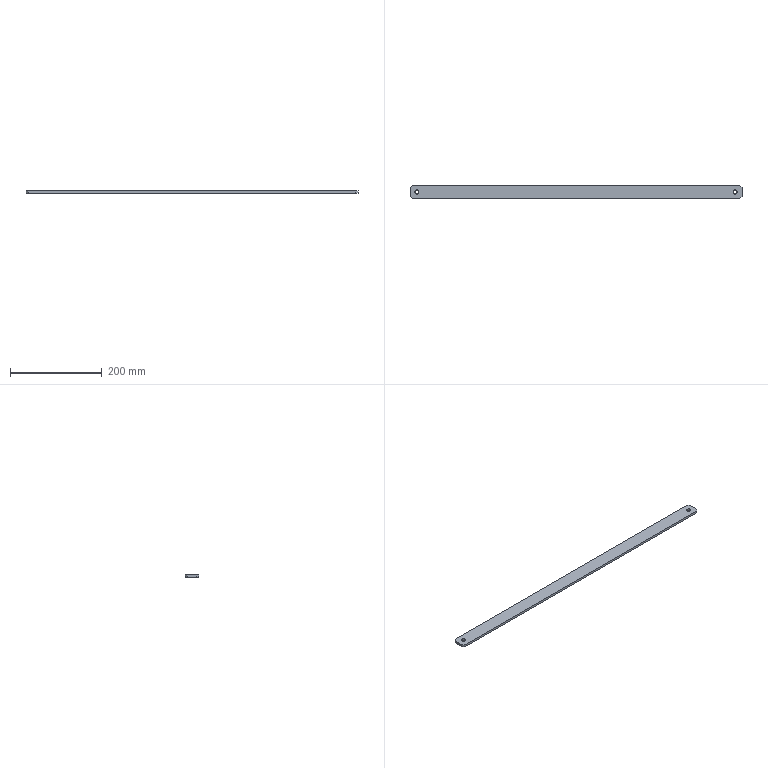Part | STEP file | link-forlegfor roller | 1 solid | 12 faces | box 725.486 x 30 x 5 mm | volume 107937 mm3 | plane 10 | spline 2
STEP:
#1=CARTESIAN_POINT('',(0.,0.,0.));
#2=DIRECTION('',(0.,0.,1.));
#3=DIRECTION('',(1.,0.,0.));
#4=AXIS2_PLACEMENT_3D('',#1,#2,#3);
#5=CARTESIAN_POINT('',(705.986,15.,0.));
#6=VERTEX_POINT('',#5);
#7=CARTESIAN_POINT('',(710.486,15.,0.));
#8=DIRECTION('',(0.,0.,1.));
#9=DIRECTION('',(1.,0.,0.));
#10=AXIS2_PLACEMENT_3D('',#7,#8,#9);
#11=CIRCLE('',#10,4.5);
#12=CARTESIAN_POINT('',(705.986,15.,5.));
#13=CARTESIAN_POINT('',(705.986,10.5,5.));
#14=CARTESIAN_POINT('',(710.486,10.5,5.));
#15=CARTESIAN_POINT('',(714.986,10.5,5.));
#16=CARTESIAN_POINT('',(714.986,15.,5.));
#17=CARTESIAN_POINT('',(714.986,19.5,5.));
#18=CARTESIAN_POINT('',(710.486,19.5,5.));
#19=CARTESIAN_POINT('',(705.986,19.5,5.));
#20=CARTESIAN_POINT('',(705.986,15.,5.));
#21=CARTESIAN_POINT('',(705.986,15.,0.));
#22=CARTESIAN_POINT('',(705.986,10.5,0.));
#23=CARTESIAN_POINT('',(710.486,10.5,0.));
#24=CARTESIAN_POINT('',(714.986,10.5,0.));
#25=CARTESIAN_POINT('',(714.986,15.,0.));
#26=CARTESIAN_POINT('',(714.986,19.5,0.));
#27=CARTESIAN_POINT('',(710.486,19.5,0.));
#28=CARTESIAN_POINT('',(705.986,19.5,0.));
#29=CARTESIAN_POINT('',(705.986,15.,0.));
#30=(BOUNDED_SURFACE()B_SPLINE_SURFACE(1,2,((#12,#13,#14,#15,#16,#17,#18,#19,#20),(#21,#22,#23,#24,#25,#26,#27,#28,#29)),.UNSPECIFIED.,.F.,.T.,.F.)B_SPLINE_SURFACE_WITH_KNOTS((2,2),(1,2,2,2,2,2,1),(-161.361,-160.25),(-7.069,0.,7.069,14.137,21.206,28.274,35.343),.UNSPECIFIED.)GEOMETRIC_REPRESENTATION_ITEM()RATIONAL_B_SPLINE_SURFACE(((1.,0.7071,1.,0.7071,1.,0.7071,1.,0.7071,1.),(1.,0.7071,1.,0.7071,1.,0.7071,1.,0.7071,1.)))REPRESENTATION_ITEM('')SURFACE());
#31=CARTESIAN_POINT('',(-160.25,0.));
#32=CARTESIAN_POINT('',(-160.25,0.4746));
#33=CARTESIAN_POINT('',(-160.25,1.373));
#34=CARTESIAN_POINT('',(-160.25,2.623));
#35=CARTESIAN_POINT('',(-160.25,3.837));
#36=CARTESIAN_POINT('',(-160.25,5.064));
#37=CARTESIAN_POINT('',(-160.25,6.348));
#38=CARTESIAN_POINT('',(-160.25,7.789));
#39=CARTESIAN_POINT('',(-160.25,9.073));
#40=CARTESIAN_POINT('',(-160.25,10.3));
#41=CARTESIAN_POINT('',(-160.25,11.516));
#42=CARTESIAN_POINT('',(-160.25,12.758));
#43=CARTESIAN_POINT('',(-160.25,14.137));
#44=CARTESIAN_POINT('',(-160.25,15.517));
#45=CARTESIAN_POINT('',(-160.25,16.758));
#46=CARTESIAN_POINT('',(-160.25,17.974));
#47=CARTESIAN_POINT('',(-160.25,19.202));
#48=CARTESIAN_POINT('',(-160.25,20.485));
#49=CARTESIAN_POINT('',(-160.25,21.926));
#50=CARTESIAN_POINT('',(-160.25,23.21));
#51=CARTESIAN_POINT('',(-160.25,24.438));
#52=CARTESIAN_POINT('',(-160.25,25.651));
#53=CARTESIAN_POINT('',(-160.25,26.902));
#54=CARTESIAN_POINT('',(-160.25,27.8));
#55=CARTESIAN_POINT('',(-160.25,28.274));
#56=B_SPLINE_CURVE_WITH_KNOTS('',3,(#31,#32,#33,#34,#35,#36,#37,#38,#39,#40,#41,#42,#43,#44,#45,#46,#47,#48,#49,#50,#51,#52,#53,#54,#55),.UNSPECIFIED.,.F.,.F.,(4,1,1,1,1,1,1,1,1,1,1,1,1,1,1,1,1,1,1,1,1,1,4),(3.142,3.427,3.713,3.998,4.284,4.57,4.855,5.141,5.426,5.712,5.998,6.283,6.569,6.854,7.14,7.426,7.711,7.997,8.282,8.568,8.854,9.139,9.425),.QUASI_UNIFORM_KNOTS.);
#57=(GEOMETRIC_REPRESENTATION_CONTEXT(2)PARAMETRIC_REPRESENTATION_CONTEXT()REPRESENTATION_CONTEXT('',''));
#58=DEFINITIONAL_REPRESENTATION('',(#56),#57);
#59=PCURVE('',#30,#58);
#60=CARTESIAN_POINT('',(362.743,15.,0.));
#61=DIRECTION('',(0.,0.,1.));
#62=DIRECTION('',(1.,0.,0.));
#63=AXIS2_PLACEMENT_3D('',#60,#61,#62);
#64=PLANE('',#63);
#65=CARTESIAN_POINT('',(347.743,0.));
#66=DIRECTION('',(1.,0.));
#67=AXIS2_PLACEMENT_2D('',#65,#66);
#68=CIRCLE('',#67,4.5);
#69=(GEOMETRIC_REPRESENTATION_CONTEXT(2)PARAMETRIC_REPRESENTATION_CONTEXT()REPRESENTATION_CONTEXT('',''));
#70=DEFINITIONAL_REPRESENTATION('',(#68),#69);
#71=PCURVE('',#64,#70);
#72=SURFACE_CURVE('',#11,(#59,#71),.PCURVE_S1.);
#73=EDGE_CURVE('',#6,#6,#72,.T.);
#74=ORIENTED_EDGE('',*,*,#73,.T.);
#75=CARTESIAN_POINT('',(705.986,15.,5.));
#76=VERTEX_POINT('',#75);
#77=CARTESIAN_POINT('',(705.986,15.,5.));
#78=CARTESIAN_POINT('',(705.986,15.,0.));
#79=B_SPLINE_CURVE_WITH_KNOTS('',1,(#77,#78),.UNSPECIFIED.,.F.,.F.,(2,2),(-161.361,-160.25),.PIECEWISE_BEZIER_KNOTS.);
#80=CARTESIAN_POINT('',(0.,28.274));
#81=DIRECTION('',(1.,0.));
#82=VECTOR('',#81,1.);
#83=LINE('',#80,#82);
#84=(GEOMETRIC_REPRESENTATION_CONTEXT(2)PARAMETRIC_REPRESENTATION_CONTEXT()REPRESENTATION_CONTEXT('',''));
#85=DEFINITIONAL_REPRESENTATION('',(#83),#84);
#86=PCURVE('',#30,#85);
#87=CARTESIAN_POINT('',(0.,0.));
#88=DIRECTION('',(1.,0.));
#89=VECTOR('',#88,1.);
#90=LINE('',#87,#89);
#91=(GEOMETRIC_REPRESENTATION_CONTEXT(2)PARAMETRIC_REPRESENTATION_CONTEXT()REPRESENTATION_CONTEXT('',''));
#92=DEFINITIONAL_REPRESENTATION('',(#90),#91);
#93=PCURVE('',#30,#92);
#94=SEAM_CURVE('',#79,(#86,#93),.PCURVE_S1.);
#95=EDGE_CURVE('',#76,#6,#94,.T.);
#96=ORIENTED_EDGE('',*,*,#95,.F.);
#97=CARTESIAN_POINT('',(714.986,15.,5.));
#98=VERTEX_POINT('',#97);
#99=CARTESIAN_POINT('',(710.486,15.,5.));
#100=DIRECTION('',(0.,0.,-1.));
#101=DIRECTION('',(1.,0.,0.));
#102=AXIS2_PLACEMENT_3D('',#99,#100,#101);
#103=CIRCLE('',#102,4.5);
#104=CARTESIAN_POINT('',(-161.361,42.412));
#105=CARTESIAN_POINT('',(-161.361,41.937));
#106=CARTESIAN_POINT('',(-161.361,41.039));
#107=CARTESIAN_POINT('',(-161.361,39.788));
#108=CARTESIAN_POINT('',(-161.361,38.575));
#109=CARTESIAN_POINT('',(-161.361,37.347));
#110=CARTESIAN_POINT('',(-161.361,36.064));
#111=CARTESIAN_POINT('',(-161.361,34.622));
#112=CARTESIAN_POINT('',(-161.361,33.339));
#113=CARTESIAN_POINT('',(-161.361,32.111));
#114=CARTESIAN_POINT('',(-161.361,30.896));
#115=CARTESIAN_POINT('',(-161.361,29.654));
#116=CARTESIAN_POINT('',(-161.361,28.274));
#117=CARTESIAN_POINT('',(-161.361,26.895));
#118=CARTESIAN_POINT('',(-161.361,25.653));
#119=CARTESIAN_POINT('',(-161.361,24.437));
#120=CARTESIAN_POINT('',(-161.361,23.21));
#121=CARTESIAN_POINT('',(-161.361,21.926));
#122=CARTESIAN_POINT('',(-161.361,20.485));
#123=CARTESIAN_POINT('',(-161.361,19.202));
#124=CARTESIAN_POINT('',(-161.361,17.974));
#125=CARTESIAN_POINT('',(-161.361,16.76));
#126=CARTESIAN_POINT('',(-161.361,15.51));
#127=CARTESIAN_POINT('',(-161.361,14.612));
#128=CARTESIAN_POINT('',(-161.361,14.137));
#129=B_SPLINE_CURVE_WITH_KNOTS('',3,(#104,#105,#106,#107,#108,#109,#110,#111,#112,#113,#114,#115,#116,#117,#118,#119,#120,#121,#122,#123,#124,#125,#126,#127,#128),.UNSPECIFIED.,.F.,.F.,(4,1,1,1,1,1,1,1,1,1,1,1,1,1,1,1,1,1,1,1,1,1,4),(0.,0.2856,0.5712,0.8568,1.142,1.428,1.714,1.999,2.285,2.57,2.856,3.142,3.427,3.713,3.998,4.284,4.57,4.855,5.141,5.426,5.712,5.998,6.283),.QUASI_UNIFORM_KNOTS.);
#130=(GEOMETRIC_REPRESENTATION_CONTEXT(2)PARAMETRIC_REPRESENTATION_CONTEXT()REPRESENTATION_CONTEXT('',''));
#131=DEFINITIONAL_REPRESENTATION('',(#129),#130);
#132=PCURVE('',#30,#131);
#133=CARTESIAN_POINT('',(362.743,15.,5.));
#134=DIRECTION('',(0.,0.,1.));
#135=DIRECTION('',(1.,0.,0.));
#136=AXIS2_PLACEMENT_3D('',#133,#134,#135);
#137=PLANE('',#136);
#138=CARTESIAN_POINT('',(352.243,0.));
#139=CARTESIAN_POINT('',(352.243,-7.794));
#140=CARTESIAN_POINT('',(345.493,-3.897));
#141=CARTESIAN_POINT('',(338.743,0.));
#142=CARTESIAN_POINT('',(345.493,3.897));
#143=CARTESIAN_POINT('',(352.243,7.794));
#144=CARTESIAN_POINT('',(352.243,0.));
#145=(BOUNDED_CURVE()B_SPLINE_CURVE(2,(#138,#139,#140,#141,#142,#143,#144),.UNSPECIFIED.,.T.,.F.)B_SPLINE_CURVE_WITH_KNOTS((1,2,2,2,2,1),(-2.094,0.,2.094,4.189,6.283,8.378),.UNSPECIFIED.)CURVE()GEOMETRIC_REPRESENTATION_ITEM()RATIONAL_B_SPLINE_CURVE((1.,0.5,1.,0.5,1.,0.5,1.))REPRESENTATION_ITEM(''));
#146=(GEOMETRIC_REPRESENTATION_CONTEXT(2)PARAMETRIC_REPRESENTATION_CONTEXT()REPRESENTATION_CONTEXT('',''));
#147=DEFINITIONAL_REPRESENTATION('',(#145),#146);
#148=PCURVE('',#137,#147);
#149=SURFACE_CURVE('',#103,(#132,#148),.PCURVE_S1.);
#150=EDGE_CURVE('',#76,#98,#149,.T.);
#151=ORIENTED_EDGE('',*,*,#150,.T.);
#152=CARTESIAN_POINT('',(710.486,15.,5.));
#153=DIRECTION('',(0.,0.,-1.));
#154=DIRECTION('',(1.,0.,0.));
#155=AXIS2_PLACEMENT_3D('',#152,#153,#154);
#156=CIRCLE('',#155,4.5);
#157=CARTESIAN_POINT('',(-161.361,14.137));
#158=CARTESIAN_POINT('',(-161.361,13.663));
#159=CARTESIAN_POINT('',(-161.361,12.765));
#160=CARTESIAN_POINT('',(-161.361,11.514));
#161=CARTESIAN_POINT('',(-161.361,10.301));
#162=CARTESIAN_POINT('',(-161.361,9.073));
#163=CARTESIAN_POINT('',(-161.361,7.789));
#164=CARTESIAN_POINT('',(-161.361,6.348));
#165=CARTESIAN_POINT('',(-161.361,5.064));
#166=CARTESIAN_POINT('',(-161.361,3.837));
#167=CARTESIAN_POINT('',(-161.361,2.621));
#168=CARTESIAN_POINT('',(-161.361,1.379));
#169=CARTESIAN_POINT('',(-161.361,0.));
#170=CARTESIAN_POINT('',(-161.361,-1.379));
#171=CARTESIAN_POINT('',(-161.361,-2.621));
#172=CARTESIAN_POINT('',(-161.361,-3.837));
#173=CARTESIAN_POINT('',(-161.361,-5.064));
#174=CARTESIAN_POINT('',(-161.361,-6.348));
#175=CARTESIAN_POINT('',(-161.361,-7.789));
#176=CARTESIAN_POINT('',(-161.361,-9.073));
#177=CARTESIAN_POINT('',(-161.361,-10.301));
#178=CARTESIAN_POINT('',(-161.361,-11.514));
#179=CARTESIAN_POINT('',(-161.361,-12.765));
#180=CARTESIAN_POINT('',(-161.361,-13.663));
#181=CARTESIAN_POINT('',(-161.361,-14.137));
#182=B_SPLINE_CURVE_WITH_KNOTS('',3,(#157,#158,#159,#160,#161,#162,#163,#164,#165,#166,#167,#168,#169,#170,#171,#172,#173,#174,#175,#176,#177,#178,#179,#180,#181),.UNSPECIFIED.,.F.,.F.,(4,1,1,1,1,1,1,1,1,1,1,1,1,1,1,1,1,1,1,1,1,1,4),(0.,0.2856,0.5712,0.8568,1.142,1.428,1.714,1.999,2.285,2.57,2.856,3.142,3.427,3.713,3.998,4.284,4.57,4.855,5.141,5.426,5.712,5.998,6.283),.QUASI_UNIFORM_KNOTS.);
#183=(GEOMETRIC_REPRESENTATION_CONTEXT(2)PARAMETRIC_REPRESENTATION_CONTEXT()REPRESENTATION_CONTEXT('',''));
#184=DEFINITIONAL_REPRESENTATION('',(#182),#183);
#185=PCURVE('',#30,#184);
#186=CARTESIAN_POINT('',(352.243,0.));
#187=CARTESIAN_POINT('',(352.243,-7.794));
#188=CARTESIAN_POINT('',(345.493,-3.897));
#189=CARTESIAN_POINT('',(338.743,0.));
#190=CARTESIAN_POINT('',(345.493,3.897));
#191=CARTESIAN_POINT('',(352.243,7.794));
#192=CARTESIAN_POINT('',(352.243,0.));
#193=(BOUNDED_CURVE()B_SPLINE_CURVE(2,(#186,#187,#188,#189,#190,#191,#192),.UNSPECIFIED.,.T.,.F.)B_SPLINE_CURVE_WITH_KNOTS((1,2,2,2,2,1),(-2.094,0.,2.094,4.189,6.283,8.378),.UNSPECIFIED.)CURVE()GEOMETRIC_REPRESENTATION_ITEM()RATIONAL_B_SPLINE_CURVE((1.,0.5,1.,0.5,1.,0.5,1.))REPRESENTATION_ITEM(''));
#194=(GEOMETRIC_REPRESENTATION_CONTEXT(2)PARAMETRIC_REPRESENTATION_CONTEXT()REPRESENTATION_CONTEXT('',''));
#195=DEFINITIONAL_REPRESENTATION('',(#193),#194);
#196=PCURVE('',#137,#195);
#197=SURFACE_CURVE('',#156,(#185,#196),.PCURVE_S1.);
#198=EDGE_CURVE('',#98,#76,#197,.T.);
#199=ORIENTED_EDGE('',*,*,#198,.T.);
#200=ORIENTED_EDGE('',*,*,#95,.T.);
#201=EDGE_LOOP('',(#74,#96,#151,#199,#200));
#202=FACE_BOUND('',#201,.F.);
#203=ADVANCED_FACE('',(#202),#30,.F.);
#204=CARTESIAN_POINT('',(10.5,15.,0.));
#205=VERTEX_POINT('',#204);
#206=CARTESIAN_POINT('',(15.,15.,0.));
#207=DIRECTION('',(0.,0.,1.));
#208=DIRECTION('',(1.,0.,0.));
#209=AXIS2_PLACEMENT_3D('',#206,#207,#208);
#210=CIRCLE('',#209,4.5);
#211=CARTESIAN_POINT('',(10.5,15.,5.));
#212=CARTESIAN_POINT('',(10.5,10.5,5.));
#213=CARTESIAN_POINT('',(15.,10.5,5.));
#214=CARTESIAN_POINT('',(19.5,10.5,5.));
#215=CARTESIAN_POINT('',(19.5,15.,5.));
#216=CARTESIAN_POINT('',(19.5,19.5,5.));
#217=CARTESIAN_POINT('',(15.,19.5,5.));
#218=CARTESIAN_POINT('',(10.5,19.5,5.));
#219=CARTESIAN_POINT('',(10.5,15.,5.));
#220=CARTESIAN_POINT('',(10.5,15.,0.));
#221=CARTESIAN_POINT('',(10.5,10.5,0.));
#222=CARTESIAN_POINT('',(15.,10.5,0.));
#223=CARTESIAN_POINT('',(19.5,10.5,0.));
#224=CARTESIAN_POINT('',(19.5,15.,0.));
#225=CARTESIAN_POINT('',(19.5,19.5,0.));
#226=CARTESIAN_POINT('',(15.,19.5,0.));
#227=CARTESIAN_POINT('',(10.5,19.5,0.));
#228=CARTESIAN_POINT('',(10.5,15.,0.));
#229=(BOUNDED_SURFACE()B_SPLINE_SURFACE(1,2,((#211,#212,#213,#214,#215,#216,#217,#218,#219),(#220,#221,#222,#223,#224,#225,#226,#227,#228)),.UNSPECIFIED.,.F.,.T.,.F.)B_SPLINE_SURFACE_WITH_KNOTS((2,2),(1,2,2,2,2,2,1),(-161.361,-160.25),(-7.069,0.,7.069,14.137,21.206,28.274,35.343),.UNSPECIFIED.)GEOMETRIC_REPRESENTATION_ITEM()RATIONAL_B_SPLINE_SURFACE(((1.,0.7071,1.,0.7071,1.,0.7071,1.,0.7071,1.),(1.,0.7071,1.,0.7071,1.,0.7071,1.,0.7071,1.)))REPRESENTATION_ITEM('')SURFACE());
#230=CARTESIAN_POINT('',(-160.25,0.));
#231=CARTESIAN_POINT('',(-160.25,0.4746));
#232=CARTESIAN_POINT('',(-160.25,1.373));
#233=CARTESIAN_POINT('',(-160.25,2.623));
#234=CARTESIAN_POINT('',(-160.25,3.837));
#235=CARTESIAN_POINT('',(-160.25,5.064));
#236=CARTESIAN_POINT('',(-160.25,6.348));
#237=CARTESIAN_POINT('',(-160.25,7.789));
#238=CARTESIAN_POINT('',(-160.25,9.073));
#239=CARTESIAN_POINT('',(-160.25,10.3));
#240=CARTESIAN_POINT('',(-160.25,11.516));
#241=CARTESIAN_POINT('',(-160.25,12.758));
#242=CARTESIAN_POINT('',(-160.25,14.137));
#243=CARTESIAN_POINT('',(-160.25,15.517));
#244=CARTESIAN_POINT('',(-160.25,16.758));
#245=CARTESIAN_POINT('',(-160.25,17.974));
#246=CARTESIAN_POINT('',(-160.25,19.202));
#247=CARTESIAN_POINT('',(-160.25,20.485));
#248=CARTESIAN_POINT('',(-160.25,21.926));
#249=CARTESIAN_POINT('',(-160.25,23.21));
#250=CARTESIAN_POINT('',(-160.25,24.438));
#251=CARTESIAN_POINT('',(-160.25,25.651));
#252=CARTESIAN_POINT('',(-160.25,26.902));
#253=CARTESIAN_POINT('',(-160.25,27.8));
#254=CARTESIAN_POINT('',(-160.25,28.274));
#255=B_SPLINE_CURVE_WITH_KNOTS('',3,(#230,#231,#232,#233,#234,#235,#236,#237,#238,#239,#240,#241,#242,#243,#244,#245,#246,#247,#248,#249,#250,#251,#252,#253,#254),.UNSPECIFIED.,.F.,.F.,(4,1,1,1,1,1,1,1,1,1,1,1,1,1,1,1,1,1,1,1,1,1,4),(3.142,3.427,3.713,3.998,4.284,4.57,4.855,5.141,5.426,5.712,5.998,6.283,6.569,6.854,7.14,7.426,7.711,7.997,8.282,8.568,8.854,9.139,9.425),.QUASI_UNIFORM_KNOTS.);
#256=(GEOMETRIC_REPRESENTATION_CONTEXT(2)PARAMETRIC_REPRESENTATION_CONTEXT()REPRESENTATION_CONTEXT('',''));
#257=DEFINITIONAL_REPRESENTATION('',(#255),#256);
#258=PCURVE('',#229,#257);
#259=CARTESIAN_POINT('',(-347.743,0.));
#260=DIRECTION('',(1.,0.));
#261=AXIS2_PLACEMENT_2D('',#259,#260);
#262=CIRCLE('',#261,4.5);
#263=(GEOMETRIC_REPRESENTATION_CONTEXT(2)PARAMETRIC_REPRESENTATION_CONTEXT()REPRESENTATION_CONTEXT('',''));
#264=DEFINITIONAL_REPRESENTATION('',(#262),#263);
#265=PCURVE('',#64,#264);
#266=SURFACE_CURVE('',#210,(#258,#265),.PCURVE_S1.);
#267=EDGE_CURVE('',#205,#205,#266,.T.);
#268=ORIENTED_EDGE('',*,*,#267,.T.);
#269=CARTESIAN_POINT('',(10.5,15.,5.));
#270=VERTEX_POINT('',#269);
#271=CARTESIAN_POINT('',(10.5,15.,5.));
#272=CARTESIAN_POINT('',(10.5,15.,0.));
#273=B_SPLINE_CURVE_WITH_KNOTS('',1,(#271,#272),.UNSPECIFIED.,.F.,.F.,(2,2),(-161.361,-160.25),.PIECEWISE_BEZIER_KNOTS.);
#274=CARTESIAN_POINT('',(0.,28.274));
#275=DIRECTION('',(1.,0.));
#276=VECTOR('',#275,1.);
#277=LINE('',#274,#276);
#278=(GEOMETRIC_REPRESENTATION_CONTEXT(2)PARAMETRIC_REPRESENTATION_CONTEXT()REPRESENTATION_CONTEXT('',''));
#279=DEFINITIONAL_REPRESENTATION('',(#277),#278);
#280=PCURVE('',#229,#279);
#281=CARTESIAN_POINT('',(0.,0.));
#282=DIRECTION('',(1.,0.));
#283=VECTOR('',#282,1.);
#284=LINE('',#281,#283);
#285=(GEOMETRIC_REPRESENTATION_CONTEXT(2)PARAMETRIC_REPRESENTATION_CONTEXT()REPRESENTATION_CONTEXT('',''));
#286=DEFINITIONAL_REPRESENTATION('',(#284),#285);
#287=PCURVE('',#229,#286);
#288=SEAM_CURVE('',#273,(#280,#287),.PCURVE_S1.);
#289=EDGE_CURVE('',#270,#205,#288,.T.);
#290=ORIENTED_EDGE('',*,*,#289,.F.);
#291=CARTESIAN_POINT('',(19.5,15.,5.));
#292=VERTEX_POINT('',#291);
#293=CARTESIAN_POINT('',(15.,15.,5.));
#294=DIRECTION('',(0.,0.,-1.));
#295=DIRECTION('',(1.,0.,0.));
#296=AXIS2_PLACEMENT_3D('',#293,#294,#295);
#297=CIRCLE('',#296,4.5);
#298=CARTESIAN_POINT('',(-161.361,42.412));
#299=CARTESIAN_POINT('',(-161.361,41.937));
#300=CARTESIAN_POINT('',(-161.361,41.039));
#301=CARTESIAN_POINT('',(-161.361,39.788));
#302=CARTESIAN_POINT('',(-161.361,38.575));
#303=CARTESIAN_POINT('',(-161.361,37.347));
#304=CARTESIAN_POINT('',(-161.361,36.064));
#305=CARTESIAN_POINT('',(-161.361,34.622));
#306=CARTESIAN_POINT('',(-161.361,33.339));
#307=CARTESIAN_POINT('',(-161.361,32.111));
#308=CARTESIAN_POINT('',(-161.361,30.896));
#309=CARTESIAN_POINT('',(-161.361,29.654));
#310=CARTESIAN_POINT('',(-161.361,28.274));
#311=CARTESIAN_POINT('',(-161.361,26.895));
#312=CARTESIAN_POINT('',(-161.361,25.653));
#313=CARTESIAN_POINT('',(-161.361,24.437));
#314=CARTESIAN_POINT('',(-161.361,23.21));
#315=CARTESIAN_POINT('',(-161.361,21.926));
#316=CARTESIAN_POINT('',(-161.361,20.485));
#317=CARTESIAN_POINT('',(-161.361,19.202));
#318=CARTESIAN_POINT('',(-161.361,17.974));
#319=CARTESIAN_POINT('',(-161.361,16.76));
#320=CARTESIAN_POINT('',(-161.361,15.51));
#321=CARTESIAN_POINT('',(-161.361,14.612));
#322=CARTESIAN_POINT('',(-161.361,14.137));
#323=B_SPLINE_CURVE_WITH_KNOTS('',3,(#298,#299,#300,#301,#302,#303,#304,#305,#306,#307,#308,#309,#310,#311,#312,#313,#314,#315,#316,#317,#318,#319,#320,#321,#322),.UNSPECIFIED.,.F.,.F.,(4,1,1,1,1,1,1,1,1,1,1,1,1,1,1,1,1,1,1,1,1,1,4),(0.,0.2856,0.5712,0.8568,1.142,1.428,1.714,1.999,2.285,2.57,2.856,3.142,3.427,3.713,3.998,4.284,4.57,4.855,5.141,5.426,5.712,5.998,6.283),.QUASI_UNIFORM_KNOTS.);
#324=(GEOMETRIC_REPRESENTATION_CONTEXT(2)PARAMETRIC_REPRESENTATION_CONTEXT()REPRESENTATION_CONTEXT('',''));
#325=DEFINITIONAL_REPRESENTATION('',(#323),#324);
#326=PCURVE('',#229,#325);
#327=CARTESIAN_POINT('',(-343.243,0.));
#328=CARTESIAN_POINT('',(-343.243,-7.794));
#329=CARTESIAN_POINT('',(-349.993,-3.897));
#330=CARTESIAN_POINT('',(-356.743,0.));
#331=CARTESIAN_POINT('',(-349.993,3.897));
#332=CARTESIAN_POINT('',(-343.243,7.794));
#333=CARTESIAN_POINT('',(-343.243,0.));
#334=(BOUNDED_CURVE()B_SPLINE_CURVE(2,(#327,#328,#329,#330,#331,#332,#333),.UNSPECIFIED.,.T.,.F.)B_SPLINE_CURVE_WITH_KNOTS((1,2,2,2,2,1),(-2.094,0.,2.094,4.189,6.283,8.378),.UNSPECIFIED.)CURVE()GEOMETRIC_REPRESENTATION_ITEM()RATIONAL_B_SPLINE_CURVE((1.,0.5,1.,0.5,1.,0.5,1.))REPRESENTATION_ITEM(''));
#335=(GEOMETRIC_REPRESENTATION_CONTEXT(2)PARAMETRIC_REPRESENTATION_CONTEXT()REPRESENTATION_CONTEXT('',''));
#336=DEFINITIONAL_REPRESENTATION('',(#334),#335);
#337=PCURVE('',#137,#336);
#338=SURFACE_CURVE('',#297,(#326,#337),.PCURVE_S1.);
#339=EDGE_CURVE('',#270,#292,#338,.T.);
#340=ORIENTED_EDGE('',*,*,#339,.T.);
#341=CARTESIAN_POINT('',(15.,15.,5.));
#342=DIRECTION('',(0.,0.,-1.));
#343=DIRECTION('',(1.,0.,0.));
#344=AXIS2_PLACEMENT_3D('',#341,#342,#343);
#345=CIRCLE('',#344,4.5);
#346=CARTESIAN_POINT('',(-161.361,14.137));
#347=CARTESIAN_POINT('',(-161.361,13.663));
#348=CARTESIAN_POINT('',(-161.361,12.765));
#349=CARTESIAN_POINT('',(-161.361,11.514));
#350=CARTESIAN_POINT('',(-161.361,10.301));
#351=CARTESIAN_POINT('',(-161.361,9.073));
#352=CARTESIAN_POINT('',(-161.361,7.789));
#353=CARTESIAN_POINT('',(-161.361,6.348));
#354=CARTESIAN_POINT('',(-161.361,5.064));
#355=CARTESIAN_POINT('',(-161.361,3.837));
#356=CARTESIAN_POINT('',(-161.361,2.621));
#357=CARTESIAN_POINT('',(-161.361,1.379));
#358=CARTESIAN_POINT('',(-161.361,0.));
#359=CARTESIAN_POINT('',(-161.361,-1.379));
#360=CARTESIAN_POINT('',(-161.361,-2.621));
#361=CARTESIAN_POINT('',(-161.361,-3.837));
#362=CARTESIAN_POINT('',(-161.361,-5.064));
#363=CARTESIAN_POINT('',(-161.361,-6.348));
#364=CARTESIAN_POINT('',(-161.361,-7.789));
#365=CARTESIAN_POINT('',(-161.361,-9.073));
#366=CARTESIAN_POINT('',(-161.361,-10.301));
#367=CARTESIAN_POINT('',(-161.361,-11.514));
#368=CARTESIAN_POINT('',(-161.361,-12.765));
#369=CARTESIAN_POINT('',(-161.361,-13.663));
#370=CARTESIAN_POINT('',(-161.361,-14.137));
#371=B_SPLINE_CURVE_WITH_KNOTS('',3,(#346,#347,#348,#349,#350,#351,#352,#353,#354,#355,#356,#357,#358,#359,#360,#361,#362,#363,#364,#365,#366,#367,#368,#369,#370),.UNSPECIFIED.,.F.,.F.,(4,1,1,1,1,1,1,1,1,1,1,1,1,1,1,1,1,1,1,1,1,1,4),(0.,0.2856,0.5712,0.8568,1.142,1.428,1.714,1.999,2.285,2.57,2.856,3.142,3.427,3.713,3.998,4.284,4.57,4.855,5.141,5.426,5.712,5.998,6.283),.QUASI_UNIFORM_KNOTS.);
#372=(GEOMETRIC_REPRESENTATION_CONTEXT(2)PARAMETRIC_REPRESENTATION_CONTEXT()REPRESENTATION_CONTEXT('',''));
#373=DEFINITIONAL_REPRESENTATION('',(#371),#372);
#374=PCURVE('',#229,#373);
#375=CARTESIAN_POINT('',(-343.243,0.));
#376=CARTESIAN_POINT('',(-343.243,-7.794));
#377=CARTESIAN_POINT('',(-349.993,-3.897));
#378=CARTESIAN_POINT('',(-356.743,0.));
#379=CARTESIAN_POINT('',(-349.993,3.897));
#380=CARTESIAN_POINT('',(-343.243,7.794));
#381=CARTESIAN_POINT('',(-343.243,0.));
#382=(BOUNDED_CURVE()B_SPLINE_CURVE(2,(#375,#376,#377,#378,#379,#380,#381),.UNSPECIFIED.,.T.,.F.)B_SPLINE_CURVE_WITH_KNOTS((1,2,2,2,2,1),(-2.094,0.,2.094,4.189,6.283,8.378),.UNSPECIFIED.)CURVE()GEOMETRIC_REPRESENTATION_ITEM()RATIONAL_B_SPLINE_CURVE((1.,0.5,1.,0.5,1.,0.5,1.))REPRESENTATION_ITEM(''));
#383=(GEOMETRIC_REPRESENTATION_CONTEXT(2)PARAMETRIC_REPRESENTATION_CONTEXT()REPRESENTATION_CONTEXT('',''));
#384=DEFINITIONAL_REPRESENTATION('',(#382),#383);
#385=PCURVE('',#137,#384);
#386=SURFACE_CURVE('',#345,(#374,#385),.PCURVE_S1.);
#387=EDGE_CURVE('',#292,#270,#386,.T.);
#388=ORIENTED_EDGE('',*,*,#387,.T.);
#389=ORIENTED_EDGE('',*,*,#289,.T.);
#390=EDGE_LOOP('',(#268,#290,#340,#388,#389));
#391=FACE_BOUND('',#390,.F.);
#392=ADVANCED_FACE('',(#391),#229,.F.);
#393=CARTESIAN_POINT('',(720.486,30.,5.));
#394=VERTEX_POINT('',#393);
#395=CARTESIAN_POINT('',(725.486,25.,5.));
#396=VERTEX_POINT('',#395);
#397=CARTESIAN_POINT('',(720.486,30.,5.));
#398=DIRECTION('',(0.7071,-0.7071,0.));
#399=VECTOR('',#398,1.);
#400=LINE('',#397,#399);
#401=CARTESIAN_POINT('',(722.986,27.5,0.));
#402=DIRECTION('',(0.7071,0.7071,0.));
#403=DIRECTION('',(0.,0.,-1.));
#404=AXIS2_PLACEMENT_3D('',#401,#402,#403);
#405=PLANE('',#404);
#406=CARTESIAN_POINT('',(-5.,3.536));
#407=DIRECTION('',(0.,-1.));
#408=VECTOR('',#407,1.);
#409=LINE('',#406,#408);
#410=(GEOMETRIC_REPRESENTATION_CONTEXT(2)PARAMETRIC_REPRESENTATION_CONTEXT()REPRESENTATION_CONTEXT('',''));
#411=DEFINITIONAL_REPRESENTATION('',(#409),#410);
#412=PCURVE('',#405,#411);
#413=CARTESIAN_POINT('',(357.743,15.));
#414=DIRECTION('',(0.7071,-0.7071));
#415=VECTOR('',#414,1.);
#416=LINE('',#413,#415);
#417=(GEOMETRIC_REPRESENTATION_CONTEXT(2)PARAMETRIC_REPRESENTATION_CONTEXT()REPRESENTATION_CONTEXT('',''));
#418=DEFINITIONAL_REPRESENTATION('',(#416),#417);
#419=PCURVE('',#137,#418);
#420=SURFACE_CURVE('',#400,(#412,#419),.PCURVE_S1.);
#421=EDGE_CURVE('',#394,#396,#420,.T.);
#422=ORIENTED_EDGE('',*,*,#421,.T.);
#423=CARTESIAN_POINT('',(725.486,25.,0.));
#424=VERTEX_POINT('',#423);
#425=CARTESIAN_POINT('',(725.486,25.,5.));
#426=DIRECTION('',(0.,0.,-1.));
#427=VECTOR('',#426,1.);
#428=LINE('',#425,#427);
#429=CARTESIAN_POINT('',(-5.,-3.536));
#430=DIRECTION('',(1.,0.));
#431=VECTOR('',#430,1.);
#432=LINE('',#429,#431);
#433=(GEOMETRIC_REPRESENTATION_CONTEXT(2)PARAMETRIC_REPRESENTATION_CONTEXT()REPRESENTATION_CONTEXT('',''));
#434=DEFINITIONAL_REPRESENTATION('',(#432),#433);
#435=PCURVE('',#405,#434);
#436=CARTESIAN_POINT('',(725.486,30.,0.));
#437=DIRECTION('',(1.,0.,0.));
#438=DIRECTION('',(0.,0.,-1.));
#439=AXIS2_PLACEMENT_3D('',#436,#437,#438);
#440=PLANE('',#439);
#441=CARTESIAN_POINT('',(-5.,-5.));
#442=DIRECTION('',(1.,0.));
#443=VECTOR('',#442,1.);
#444=LINE('',#441,#443);
#445=(GEOMETRIC_REPRESENTATION_CONTEXT(2)PARAMETRIC_REPRESENTATION_CONTEXT()REPRESENTATION_CONTEXT('',''));
#446=DEFINITIONAL_REPRESENTATION('',(#444),#445);
#447=PCURVE('',#440,#446);
#448=SURFACE_CURVE('',#428,(#435,#447),.PCURVE_S1.);
#449=EDGE_CURVE('',#396,#424,#448,.T.);
#450=ORIENTED_EDGE('',*,*,#449,.T.);
#451=CARTESIAN_POINT('',(720.486,30.,0.));
#452=VERTEX_POINT('',#451);
#453=CARTESIAN_POINT('',(725.486,25.,0.));
#454=DIRECTION('',(-0.7071,0.7071,0.));
#455=VECTOR('',#454,1.);
#456=LINE('',#453,#455);
#457=CARTESIAN_POINT('',(0.,-3.536));
#458=DIRECTION('',(0.,1.));
#459=VECTOR('',#458,1.);
#460=LINE('',#457,#459);
#461=(GEOMETRIC_REPRESENTATION_CONTEXT(2)PARAMETRIC_REPRESENTATION_CONTEXT()REPRESENTATION_CONTEXT('',''));
#462=DEFINITIONAL_REPRESENTATION('',(#460),#461);
#463=PCURVE('',#405,#462);
#464=CARTESIAN_POINT('',(362.743,10.));
#465=DIRECTION('',(-0.7071,0.7071));
#466=VECTOR('',#465,1.);
#467=LINE('',#464,#466);
#468=(GEOMETRIC_REPRESENTATION_CONTEXT(2)PARAMETRIC_REPRESENTATION_CONTEXT()REPRESENTATION_CONTEXT('',''));
#469=DEFINITIONAL_REPRESENTATION('',(#467),#468);
#470=PCURVE('',#64,#469);
#471=SURFACE_CURVE('',#456,(#463,#470),.PCURVE_S1.);
#472=EDGE_CURVE('',#424,#452,#471,.T.);
#473=ORIENTED_EDGE('',*,*,#472,.T.);
#474=CARTESIAN_POINT('',(720.486,30.,0.));
#475=DIRECTION('',(0.,0.,1.));
#476=VECTOR('',#475,1.);
#477=LINE('',#474,#476);
#478=CARTESIAN_POINT('',(0.,3.536));
#479=DIRECTION('',(-1.,0.));
#480=VECTOR('',#479,1.);
#481=LINE('',#478,#480);
#482=(GEOMETRIC_REPRESENTATION_CONTEXT(2)PARAMETRIC_REPRESENTATION_CONTEXT()REPRESENTATION_CONTEXT('',''));
#483=DEFINITIONAL_REPRESENTATION('',(#481),#482);
#484=PCURVE('',#405,#483);
#485=CARTESIAN_POINT('',(0.,30.,0.));
#486=DIRECTION('',(0.,1.,0.));
#487=DIRECTION('',(0.,0.,1.));
#488=AXIS2_PLACEMENT_3D('',#485,#486,#487);
#489=PLANE('',#488);
#490=CARTESIAN_POINT('',(0.,720.486));
#491=DIRECTION('',(1.,0.));
#492=VECTOR('',#491,1.);
#493=LINE('',#490,#492);
#494=(GEOMETRIC_REPRESENTATION_CONTEXT(2)PARAMETRIC_REPRESENTATION_CONTEXT()REPRESENTATION_CONTEXT('',''));
#495=DEFINITIONAL_REPRESENTATION('',(#493),#494);
#496=PCURVE('',#489,#495);
#497=SURFACE_CURVE('',#477,(#484,#496),.PCURVE_S1.);
#498=EDGE_CURVE('',#452,#394,#497,.T.);
#499=ORIENTED_EDGE('',*,*,#498,.T.);
#500=EDGE_LOOP('',(#422,#450,#473,#499));
#501=FACE_BOUND('',#500,.T.);
#502=ADVANCED_FACE('',(#501),#405,.T.);
#503=ORIENTED_EDGE('',*,*,#421,.F.);
#504=CARTESIAN_POINT('',(5.,30.,5.));
#505=VERTEX_POINT('',#504);
#506=CARTESIAN_POINT('',(5.,30.,5.));
#507=DIRECTION('',(1.,0.,0.));
#508=VECTOR('',#507,1.);
#509=LINE('',#506,#508);
#510=CARTESIAN_POINT('',(-357.743,15.));
#511=DIRECTION('',(1.,0.));
#512=VECTOR('',#511,1.);
#513=LINE('',#510,#512);
#514=(GEOMETRIC_REPRESENTATION_CONTEXT(2)PARAMETRIC_REPRESENTATION_CONTEXT()REPRESENTATION_CONTEXT('',''));
#515=DEFINITIONAL_REPRESENTATION('',(#513),#514);
#516=PCURVE('',#137,#515);
#517=CARTESIAN_POINT('',(5.,5.));
#518=DIRECTION('',(0.,1.));
#519=VECTOR('',#518,1.);
#520=LINE('',#517,#519);
#521=(GEOMETRIC_REPRESENTATION_CONTEXT(2)PARAMETRIC_REPRESENTATION_CONTEXT()REPRESENTATION_CONTEXT('',''));
#522=DEFINITIONAL_REPRESENTATION('',(#520),#521);
#523=PCURVE('',#489,#522);
#524=SURFACE_CURVE('',#509,(#516,#523),.PCURVE_S1.);
#525=EDGE_CURVE('',#505,#394,#524,.T.);
#526=ORIENTED_EDGE('',*,*,#525,.F.);
#527=CARTESIAN_POINT('',(0.,25.,5.));
#528=VERTEX_POINT('',#527);
#529=CARTESIAN_POINT('',(0.,25.,5.));
#530=DIRECTION('',(0.7071,0.7071,0.));
#531=VECTOR('',#530,1.);
#532=LINE('',#529,#531);
#533=CARTESIAN_POINT('',(-362.743,10.));
#534=DIRECTION('',(0.7071,0.7071));
#535=VECTOR('',#534,1.);
#536=LINE('',#533,#535);
#537=(GEOMETRIC_REPRESENTATION_CONTEXT(2)PARAMETRIC_REPRESENTATION_CONTEXT()REPRESENTATION_CONTEXT('',''));
#538=DEFINITIONAL_REPRESENTATION('',(#536),#537);
#539=PCURVE('',#137,#538);
#540=CARTESIAN_POINT('',(2.5,27.5,0.));
#541=DIRECTION('',(-0.7071,0.7071,0.));
#542=DIRECTION('',(0.,0.,1.));
#543=AXIS2_PLACEMENT_3D('',#540,#541,#542);
#544=PLANE('',#543);
#545=CARTESIAN_POINT('',(5.,-3.536));
#546=DIRECTION('',(0.,1.));
#547=VECTOR('',#546,1.);
#548=LINE('',#545,#547);
#549=(GEOMETRIC_REPRESENTATION_CONTEXT(2)PARAMETRIC_REPRESENTATION_CONTEXT()REPRESENTATION_CONTEXT('',''));
#550=DEFINITIONAL_REPRESENTATION('',(#548),#549);
#551=PCURVE('',#544,#550);
#552=SURFACE_CURVE('',#532,(#539,#551),.PCURVE_S1.);
#553=EDGE_CURVE('',#528,#505,#552,.T.);
#554=ORIENTED_EDGE('',*,*,#553,.F.);
#555=CARTESIAN_POINT('',(0.,5.,5.));
#556=VERTEX_POINT('',#555);
#557=CARTESIAN_POINT('',(0.,5.,5.));
#558=DIRECTION('',(0.,1.,0.));
#559=VECTOR('',#558,1.);
#560=LINE('',#557,#559);
#561=CARTESIAN_POINT('',(-362.743,-10.));
#562=DIRECTION('',(0.,1.));
#563=VECTOR('',#562,1.);
#564=LINE('',#561,#563);
#565=(GEOMETRIC_REPRESENTATION_CONTEXT(2)PARAMETRIC_REPRESENTATION_CONTEXT()REPRESENTATION_CONTEXT('',''));
#566=DEFINITIONAL_REPRESENTATION('',(#564),#565);
#567=PCURVE('',#137,#566);
#568=CARTESIAN_POINT('',(0.,0.,0.));
#569=DIRECTION('',(-1.,0.,0.));
#570=DIRECTION('',(0.,0.,1.));
#571=AXIS2_PLACEMENT_3D('',#568,#569,#570);
#572=PLANE('',#571);
#573=CARTESIAN_POINT('',(5.,5.));
#574=DIRECTION('',(0.,1.));
#575=VECTOR('',#574,1.);
#576=LINE('',#573,#575);
#577=(GEOMETRIC_REPRESENTATION_CONTEXT(2)PARAMETRIC_REPRESENTATION_CONTEXT()REPRESENTATION_CONTEXT('',''));
#578=DEFINITIONAL_REPRESENTATION('',(#576),#577);
#579=PCURVE('',#572,#578);
#580=SURFACE_CURVE('',#560,(#567,#579),.PCURVE_S1.);
#581=EDGE_CURVE('',#556,#528,#580,.T.);
#582=ORIENTED_EDGE('',*,*,#581,.F.);
#583=CARTESIAN_POINT('',(5.,0.,5.));
#584=VERTEX_POINT('',#583);
#585=CARTESIAN_POINT('',(5.,0.,5.));
#586=DIRECTION('',(-0.7071,0.7071,0.));
#587=VECTOR('',#586,1.);
#588=LINE('',#585,#587);
#589=CARTESIAN_POINT('',(-357.743,-15.));
#590=DIRECTION('',(-0.7071,0.7071));
#591=VECTOR('',#590,1.);
#592=LINE('',#589,#591);
#593=(GEOMETRIC_REPRESENTATION_CONTEXT(2)PARAMETRIC_REPRESENTATION_CONTEXT()REPRESENTATION_CONTEXT('',''));
#594=DEFINITIONAL_REPRESENTATION('',(#592),#593);
#595=PCURVE('',#137,#594);
#596=CARTESIAN_POINT('',(2.5,2.5,0.));
#597=DIRECTION('',(-0.7071,-0.7071,0.));
#598=DIRECTION('',(0.,0.,1.));
#599=AXIS2_PLACEMENT_3D('',#596,#597,#598);
#600=PLANE('',#599);
#601=CARTESIAN_POINT('',(5.,-3.536));
#602=DIRECTION('',(0.,1.));
#603=VECTOR('',#602,1.);
#604=LINE('',#601,#603);
#605=(GEOMETRIC_REPRESENTATION_CONTEXT(2)PARAMETRIC_REPRESENTATION_CONTEXT()REPRESENTATION_CONTEXT('',''));
#606=DEFINITIONAL_REPRESENTATION('',(#604),#605);
#607=PCURVE('',#600,#606);
#608=SURFACE_CURVE('',#588,(#595,#607),.PCURVE_S1.);
#609=EDGE_CURVE('',#584,#556,#608,.T.);
#610=ORIENTED_EDGE('',*,*,#609,.F.);
#611=CARTESIAN_POINT('',(720.486,0.,5.));
#612=VERTEX_POINT('',#611);
#613=CARTESIAN_POINT('',(720.486,0.,5.));
#614=DIRECTION('',(-1.,0.,0.));
#615=VECTOR('',#614,1.);
#616=LINE('',#613,#615);
#617=CARTESIAN_POINT('',(357.743,-15.));
#618=DIRECTION('',(-1.,0.));
#619=VECTOR('',#618,1.);
#620=LINE('',#617,#619);
#621=(GEOMETRIC_REPRESENTATION_CONTEXT(2)PARAMETRIC_REPRESENTATION_CONTEXT()REPRESENTATION_CONTEXT('',''));
#622=DEFINITIONAL_REPRESENTATION('',(#620),#621);
#623=PCURVE('',#137,#622);
#624=CARTESIAN_POINT('',(725.486,0.,0.));
#625=DIRECTION('',(0.,-1.,0.));
#626=DIRECTION('',(0.,0.,-1.));
#627=AXIS2_PLACEMENT_3D('',#624,#625,#626);
#628=PLANE('',#627);
#629=CARTESIAN_POINT('',(-5.,-5.));
#630=DIRECTION('',(0.,-1.));
#631=VECTOR('',#630,1.);
#632=LINE('',#629,#631);
#633=(GEOMETRIC_REPRESENTATION_CONTEXT(2)PARAMETRIC_REPRESENTATION_CONTEXT()REPRESENTATION_CONTEXT('',''));
#634=DEFINITIONAL_REPRESENTATION('',(#632),#633);
#635=PCURVE('',#628,#634);
#636=SURFACE_CURVE('',#616,(#623,#635),.PCURVE_S1.);
#637=EDGE_CURVE('',#612,#584,#636,.T.);
#638=ORIENTED_EDGE('',*,*,#637,.F.);
#639=CARTESIAN_POINT('',(725.486,5.,5.));
#640=VERTEX_POINT('',#639);
#641=CARTESIAN_POINT('',(725.486,5.,5.));
#642=DIRECTION('',(-0.7071,-0.7071,0.));
#643=VECTOR('',#642,1.);
#644=LINE('',#641,#643);
#645=CARTESIAN_POINT('',(362.743,-10.));
#646=DIRECTION('',(-0.7071,-0.7071));
#647=VECTOR('',#646,1.);
#648=LINE('',#645,#647);
#649=(GEOMETRIC_REPRESENTATION_CONTEXT(2)PARAMETRIC_REPRESENTATION_CONTEXT()REPRESENTATION_CONTEXT('',''));
#650=DEFINITIONAL_REPRESENTATION('',(#648),#649);
#651=PCURVE('',#137,#650);
#652=CARTESIAN_POINT('',(722.986,2.5,0.));
#653=DIRECTION('',(0.7071,-0.7071,0.));
#654=DIRECTION('',(0.,0.,-1.));
#655=AXIS2_PLACEMENT_3D('',#652,#653,#654);
#656=PLANE('',#655);
#657=CARTESIAN_POINT('',(-5.,3.536));
#658=DIRECTION('',(0.,-1.));
#659=VECTOR('',#658,1.);
#660=LINE('',#657,#659);
#661=(GEOMETRIC_REPRESENTATION_CONTEXT(2)PARAMETRIC_REPRESENTATION_CONTEXT()REPRESENTATION_CONTEXT('',''));
#662=DEFINITIONAL_REPRESENTATION('',(#660),#661);
#663=PCURVE('',#656,#662);
#664=SURFACE_CURVE('',#644,(#651,#663),.PCURVE_S1.);
#665=EDGE_CURVE('',#640,#612,#664,.T.);
#666=ORIENTED_EDGE('',*,*,#665,.F.);
#667=CARTESIAN_POINT('',(725.486,25.,5.));
#668=DIRECTION('',(0.,-1.,0.));
#669=VECTOR('',#668,1.);
#670=LINE('',#667,#669);
#671=CARTESIAN_POINT('',(362.743,10.));
#672=DIRECTION('',(0.,-1.));
#673=VECTOR('',#672,1.);
#674=LINE('',#671,#673);
#675=(GEOMETRIC_REPRESENTATION_CONTEXT(2)PARAMETRIC_REPRESENTATION_CONTEXT()REPRESENTATION_CONTEXT('',''));
#676=DEFINITIONAL_REPRESENTATION('',(#674),#675);
#677=PCURVE('',#137,#676);
#678=CARTESIAN_POINT('',(-5.,-5.));
#679=DIRECTION('',(0.,-1.));
#680=VECTOR('',#679,1.);
#681=LINE('',#678,#680);
#682=(GEOMETRIC_REPRESENTATION_CONTEXT(2)PARAMETRIC_REPRESENTATION_CONTEXT()REPRESENTATION_CONTEXT('',''));
#683=DEFINITIONAL_REPRESENTATION('',(#681),#682);
#684=PCURVE('',#440,#683);
#685=SURFACE_CURVE('',#670,(#677,#684),.PCURVE_S1.);
#686=EDGE_CURVE('',#396,#640,#685,.T.);
#687=ORIENTED_EDGE('',*,*,#686,.F.);
#688=EDGE_LOOP('',(#503,#526,#554,#582,#610,#638,#666,#687));
#689=FACE_BOUND('',#688,.T.);
#690=ORIENTED_EDGE('',*,*,#198,.T.);
#691=ORIENTED_EDGE('',*,*,#150,.T.);
#692=EDGE_LOOP('',(#690,#691));
#693=FACE_BOUND('',#692,.T.);
#694=ORIENTED_EDGE('',*,*,#387,.T.);
#695=ORIENTED_EDGE('',*,*,#339,.T.);
#696=EDGE_LOOP('',(#694,#695));
#697=FACE_BOUND('',#696,.T.);
#698=ADVANCED_FACE('',(#689,#693,#697),#137,.T.);
#699=ORIENTED_EDGE('',*,*,#498,.F.);
#700=CARTESIAN_POINT('',(5.,30.,0.));
#701=VERTEX_POINT('',#700);
#702=CARTESIAN_POINT('',(720.486,30.,0.));
#703=DIRECTION('',(-1.,0.,0.));
#704=VECTOR('',#703,1.);
#705=LINE('',#702,#704);
#706=CARTESIAN_POINT('',(0.,720.486));
#707=DIRECTION('',(0.,-1.));
#708=VECTOR('',#707,1.);
#709=LINE('',#706,#708);
#710=(GEOMETRIC_REPRESENTATION_CONTEXT(2)PARAMETRIC_REPRESENTATION_CONTEXT()REPRESENTATION_CONTEXT('',''));
#711=DEFINITIONAL_REPRESENTATION('',(#709),#710);
#712=PCURVE('',#489,#711);
#713=CARTESIAN_POINT('',(357.743,15.));
#714=DIRECTION('',(-1.,0.));
#715=VECTOR('',#714,1.);
#716=LINE('',#713,#715);
#717=(GEOMETRIC_REPRESENTATION_CONTEXT(2)PARAMETRIC_REPRESENTATION_CONTEXT()REPRESENTATION_CONTEXT('',''));
#718=DEFINITIONAL_REPRESENTATION('',(#716),#717);
#719=PCURVE('',#64,#718);
#720=SURFACE_CURVE('',#705,(#712,#719),.PCURVE_S1.);
#721=EDGE_CURVE('',#452,#701,#720,.T.);
#722=ORIENTED_EDGE('',*,*,#721,.T.);
#723=CARTESIAN_POINT('',(5.,30.,5.));
#724=DIRECTION('',(0.,0.,-1.));
#725=VECTOR('',#724,1.);
#726=LINE('',#723,#725);
#727=CARTESIAN_POINT('',(5.,5.));
#728=DIRECTION('',(-1.,0.));
#729=VECTOR('',#728,1.);
#730=LINE('',#727,#729);
#731=(GEOMETRIC_REPRESENTATION_CONTEXT(2)PARAMETRIC_REPRESENTATION_CONTEXT()REPRESENTATION_CONTEXT('',''));
#732=DEFINITIONAL_REPRESENTATION('',(#730),#731);
#733=PCURVE('',#489,#732);
#734=CARTESIAN_POINT('',(5.,3.536));
#735=DIRECTION('',(-1.,0.));
#736=VECTOR('',#735,1.);
#737=LINE('',#734,#736);
#738=(GEOMETRIC_REPRESENTATION_CONTEXT(2)PARAMETRIC_REPRESENTATION_CONTEXT()REPRESENTATION_CONTEXT('',''));
#739=DEFINITIONAL_REPRESENTATION('',(#737),#738);
#740=PCURVE('',#544,#739);
#741=SURFACE_CURVE('',#726,(#733,#740),.PCURVE_S1.);
#742=EDGE_CURVE('',#505,#701,#741,.T.);
#743=ORIENTED_EDGE('',*,*,#742,.F.);
#744=ORIENTED_EDGE('',*,*,#525,.T.);
#745=EDGE_LOOP('',(#699,#722,#743,#744));
#746=FACE_BOUND('',#745,.T.);
#747=ADVANCED_FACE('',(#746),#489,.T.);
#748=ORIENTED_EDGE('',*,*,#553,.T.);
#749=ORIENTED_EDGE('',*,*,#742,.T.);
#750=CARTESIAN_POINT('',(0.,25.,0.));
#751=VERTEX_POINT('',#750);
#752=CARTESIAN_POINT('',(5.,30.,0.));
#753=DIRECTION('',(-0.7071,-0.7071,0.));
#754=VECTOR('',#753,1.);
#755=LINE('',#752,#754);
#756=CARTESIAN_POINT('',(0.,3.536));
#757=DIRECTION('',(0.,-1.));
#758=VECTOR('',#757,1.);
#759=LINE('',#756,#758);
#760=(GEOMETRIC_REPRESENTATION_CONTEXT(2)PARAMETRIC_REPRESENTATION_CONTEXT()REPRESENTATION_CONTEXT('',''));
#761=DEFINITIONAL_REPRESENTATION('',(#759),#760);
#762=PCURVE('',#544,#761);
#763=CARTESIAN_POINT('',(-357.743,15.));
#764=DIRECTION('',(-0.7071,-0.7071));
#765=VECTOR('',#764,1.);
#766=LINE('',#763,#765);
#767=(GEOMETRIC_REPRESENTATION_CONTEXT(2)PARAMETRIC_REPRESENTATION_CONTEXT()REPRESENTATION_CONTEXT('',''));
#768=DEFINITIONAL_REPRESENTATION('',(#766),#767);
#769=PCURVE('',#64,#768);
#770=SURFACE_CURVE('',#755,(#762,#769),.PCURVE_S1.);
#771=EDGE_CURVE('',#701,#751,#770,.T.);
#772=ORIENTED_EDGE('',*,*,#771,.T.);
#773=CARTESIAN_POINT('',(0.,25.,0.));
#774=DIRECTION('',(0.,0.,1.));
#775=VECTOR('',#774,1.);
#776=LINE('',#773,#775);
#777=CARTESIAN_POINT('',(0.,-3.536));
#778=DIRECTION('',(1.,0.));
#779=VECTOR('',#778,1.);
#780=LINE('',#777,#779);
#781=(GEOMETRIC_REPRESENTATION_CONTEXT(2)PARAMETRIC_REPRESENTATION_CONTEXT()REPRESENTATION_CONTEXT('',''));
#782=DEFINITIONAL_REPRESENTATION('',(#780),#781);
#783=PCURVE('',#544,#782);
#784=CARTESIAN_POINT('',(0.,25.));
#785=DIRECTION('',(1.,0.));
#786=VECTOR('',#785,1.);
#787=LINE('',#784,#786);
#788=(GEOMETRIC_REPRESENTATION_CONTEXT(2)PARAMETRIC_REPRESENTATION_CONTEXT()REPRESENTATION_CONTEXT('',''));
#789=DEFINITIONAL_REPRESENTATION('',(#787),#788);
#790=PCURVE('',#572,#789);
#791=SURFACE_CURVE('',#776,(#783,#790),.PCURVE_S1.);
#792=EDGE_CURVE('',#751,#528,#791,.T.);
#793=ORIENTED_EDGE('',*,*,#792,.T.);
#794=EDGE_LOOP('',(#748,#749,#772,#793));
#795=FACE_BOUND('',#794,.T.);
#796=ADVANCED_FACE('',(#795),#544,.T.);
#797=ORIENTED_EDGE('',*,*,#665,.T.);
#798=CARTESIAN_POINT('',(720.486,0.,0.));
#799=VERTEX_POINT('',#798);
#800=CARTESIAN_POINT('',(720.486,0.,5.));
#801=DIRECTION('',(0.,0.,-1.));
#802=VECTOR('',#801,1.);
#803=LINE('',#800,#802);
#804=CARTESIAN_POINT('',(-5.,-3.536));
#805=DIRECTION('',(1.,0.));
#806=VECTOR('',#805,1.);
#807=LINE('',#804,#806);
#808=(GEOMETRIC_REPRESENTATION_CONTEXT(2)PARAMETRIC_REPRESENTATION_CONTEXT()REPRESENTATION_CONTEXT('',''));
#809=DEFINITIONAL_REPRESENTATION('',(#807),#808);
#810=PCURVE('',#656,#809);
#811=CARTESIAN_POINT('',(-5.,-5.));
#812=DIRECTION('',(1.,0.));
#813=VECTOR('',#812,1.);
#814=LINE('',#811,#813);
#815=(GEOMETRIC_REPRESENTATION_CONTEXT(2)PARAMETRIC_REPRESENTATION_CONTEXT()REPRESENTATION_CONTEXT('',''));
#816=DEFINITIONAL_REPRESENTATION('',(#814),#815);
#817=PCURVE('',#628,#816);
#818=SURFACE_CURVE('',#803,(#810,#817),.PCURVE_S1.);
#819=EDGE_CURVE('',#612,#799,#818,.T.);
#820=ORIENTED_EDGE('',*,*,#819,.T.);
#821=CARTESIAN_POINT('',(725.486,5.,0.));
#822=VERTEX_POINT('',#821);
#823=CARTESIAN_POINT('',(720.486,0.,0.));
#824=DIRECTION('',(0.7071,0.7071,0.));
#825=VECTOR('',#824,1.);
#826=LINE('',#823,#825);
#827=CARTESIAN_POINT('',(0.,-3.536));
#828=DIRECTION('',(0.,1.));
#829=VECTOR('',#828,1.);
#830=LINE('',#827,#829);
#831=(GEOMETRIC_REPRESENTATION_CONTEXT(2)PARAMETRIC_REPRESENTATION_CONTEXT()REPRESENTATION_CONTEXT('',''));
#832=DEFINITIONAL_REPRESENTATION('',(#830),#831);
#833=PCURVE('',#656,#832);
#834=CARTESIAN_POINT('',(357.743,-15.));
#835=DIRECTION('',(0.7071,0.7071));
#836=VECTOR('',#835,1.);
#837=LINE('',#834,#836);
#838=(GEOMETRIC_REPRESENTATION_CONTEXT(2)PARAMETRIC_REPRESENTATION_CONTEXT()REPRESENTATION_CONTEXT('',''));
#839=DEFINITIONAL_REPRESENTATION('',(#837),#838);
#840=PCURVE('',#64,#839);
#841=SURFACE_CURVE('',#826,(#833,#840),.PCURVE_S1.);
#842=EDGE_CURVE('',#799,#822,#841,.T.);
#843=ORIENTED_EDGE('',*,*,#842,.T.);
#844=CARTESIAN_POINT('',(725.486,5.,0.));
#845=DIRECTION('',(0.,0.,1.));
#846=VECTOR('',#845,1.);
#847=LINE('',#844,#846);
#848=CARTESIAN_POINT('',(0.,3.536));
#849=DIRECTION('',(-1.,0.));
#850=VECTOR('',#849,1.);
#851=LINE('',#848,#850);
#852=(GEOMETRIC_REPRESENTATION_CONTEXT(2)PARAMETRIC_REPRESENTATION_CONTEXT()REPRESENTATION_CONTEXT('',''));
#853=DEFINITIONAL_REPRESENTATION('',(#851),#852);
#854=PCURVE('',#656,#853);
#855=CARTESIAN_POINT('',(0.,-25.));
#856=DIRECTION('',(-1.,0.));
#857=VECTOR('',#856,1.);
#858=LINE('',#855,#857);
#859=(GEOMETRIC_REPRESENTATION_CONTEXT(2)PARAMETRIC_REPRESENTATION_CONTEXT()REPRESENTATION_CONTEXT('',''));
#860=DEFINITIONAL_REPRESENTATION('',(#858),#859);
#861=PCURVE('',#440,#860);
#862=SURFACE_CURVE('',#847,(#854,#861),.PCURVE_S1.);
#863=EDGE_CURVE('',#822,#640,#862,.T.);
#864=ORIENTED_EDGE('',*,*,#863,.T.);
#865=EDGE_LOOP('',(#797,#820,#843,#864));
#866=FACE_BOUND('',#865,.T.);
#867=ADVANCED_FACE('',(#866),#656,.T.);
#868=ORIENTED_EDGE('',*,*,#819,.F.);
#869=ORIENTED_EDGE('',*,*,#637,.T.);
#870=CARTESIAN_POINT('',(5.,0.,0.));
#871=VERTEX_POINT('',#870);
#872=CARTESIAN_POINT('',(5.,0.,0.));
#873=DIRECTION('',(0.,0.,1.));
#874=VECTOR('',#873,1.);
#875=LINE('',#872,#874);
#876=CARTESIAN_POINT('',(0.,-720.486));
#877=DIRECTION('',(-1.,0.));
#878=VECTOR('',#877,1.);
#879=LINE('',#876,#878);
#880=(GEOMETRIC_REPRESENTATION_CONTEXT(2)PARAMETRIC_REPRESENTATION_CONTEXT()REPRESENTATION_CONTEXT('',''));
#881=DEFINITIONAL_REPRESENTATION('',(#879),#880);
#882=PCURVE('',#628,#881);
#883=CARTESIAN_POINT('',(0.,-3.536));
#884=DIRECTION('',(1.,0.));
#885=VECTOR('',#884,1.);
#886=LINE('',#883,#885);
#887=(GEOMETRIC_REPRESENTATION_CONTEXT(2)PARAMETRIC_REPRESENTATION_CONTEXT()REPRESENTATION_CONTEXT('',''));
#888=DEFINITIONAL_REPRESENTATION('',(#886),#887);
#889=PCURVE('',#600,#888);
#890=SURFACE_CURVE('',#875,(#882,#889),.PCURVE_S1.);
#891=EDGE_CURVE('',#871,#584,#890,.T.);
#892=ORIENTED_EDGE('',*,*,#891,.F.);
#893=CARTESIAN_POINT('',(5.,0.,0.));
#894=DIRECTION('',(1.,0.,0.));
#895=VECTOR('',#894,1.);
#896=LINE('',#893,#895);
#897=CARTESIAN_POINT('',(0.,-720.486));
#898=DIRECTION('',(0.,1.));
#899=VECTOR('',#898,1.);
#900=LINE('',#897,#899);
#901=(GEOMETRIC_REPRESENTATION_CONTEXT(2)PARAMETRIC_REPRESENTATION_CONTEXT()REPRESENTATION_CONTEXT('',''));
#902=DEFINITIONAL_REPRESENTATION('',(#900),#901);
#903=PCURVE('',#628,#902);
#904=CARTESIAN_POINT('',(-357.743,-15.));
#905=DIRECTION('',(1.,0.));
#906=VECTOR('',#905,1.);
#907=LINE('',#904,#906);
#908=(GEOMETRIC_REPRESENTATION_CONTEXT(2)PARAMETRIC_REPRESENTATION_CONTEXT()REPRESENTATION_CONTEXT('',''));
#909=DEFINITIONAL_REPRESENTATION('',(#907),#908);
#910=PCURVE('',#64,#909);
#911=SURFACE_CURVE('',#896,(#903,#910),.PCURVE_S1.);
#912=EDGE_CURVE('',#871,#799,#911,.T.);
#913=ORIENTED_EDGE('',*,*,#912,.T.);
#914=EDGE_LOOP('',(#868,#869,#892,#913));
#915=FACE_BOUND('',#914,.T.);
#916=ADVANCED_FACE('',(#915),#628,.T.);
#917=ORIENTED_EDGE('',*,*,#609,.T.);
#918=CARTESIAN_POINT('',(0.,5.,0.));
#919=VERTEX_POINT('',#918);
#920=CARTESIAN_POINT('',(0.,5.,5.));
#921=DIRECTION('',(0.,0.,-1.));
#922=VECTOR('',#921,1.);
#923=LINE('',#920,#922);
#924=CARTESIAN_POINT('',(5.,3.536));
#925=DIRECTION('',(-1.,0.));
#926=VECTOR('',#925,1.);
#927=LINE('',#924,#926);
#928=(GEOMETRIC_REPRESENTATION_CONTEXT(2)PARAMETRIC_REPRESENTATION_CONTEXT()REPRESENTATION_CONTEXT('',''));
#929=DEFINITIONAL_REPRESENTATION('',(#927),#928);
#930=PCURVE('',#600,#929);
#931=CARTESIAN_POINT('',(5.,5.));
#932=DIRECTION('',(-1.,0.));
#933=VECTOR('',#932,1.);
#934=LINE('',#931,#933);
#935=(GEOMETRIC_REPRESENTATION_CONTEXT(2)PARAMETRIC_REPRESENTATION_CONTEXT()REPRESENTATION_CONTEXT('',''));
#936=DEFINITIONAL_REPRESENTATION('',(#934),#935);
#937=PCURVE('',#572,#936);
#938=SURFACE_CURVE('',#923,(#930,#937),.PCURVE_S1.);
#939=EDGE_CURVE('',#556,#919,#938,.T.);
#940=ORIENTED_EDGE('',*,*,#939,.T.);
#941=CARTESIAN_POINT('',(0.,5.,0.));
#942=DIRECTION('',(0.7071,-0.7071,0.));
#943=VECTOR('',#942,1.);
#944=LINE('',#941,#943);
#945=CARTESIAN_POINT('',(0.,3.536));
#946=DIRECTION('',(0.,-1.));
#947=VECTOR('',#946,1.);
#948=LINE('',#945,#947);
#949=(GEOMETRIC_REPRESENTATION_CONTEXT(2)PARAMETRIC_REPRESENTATION_CONTEXT()REPRESENTATION_CONTEXT('',''));
#950=DEFINITIONAL_REPRESENTATION('',(#948),#949);
#951=PCURVE('',#600,#950);
#952=CARTESIAN_POINT('',(-362.743,-10.));
#953=DIRECTION('',(0.7071,-0.7071));
#954=VECTOR('',#953,1.);
#955=LINE('',#952,#954);
#956=(GEOMETRIC_REPRESENTATION_CONTEXT(2)PARAMETRIC_REPRESENTATION_CONTEXT()REPRESENTATION_CONTEXT('',''));
#957=DEFINITIONAL_REPRESENTATION('',(#955),#956);
#958=PCURVE('',#64,#957);
#959=SURFACE_CURVE('',#944,(#951,#958),.PCURVE_S1.);
#960=EDGE_CURVE('',#919,#871,#959,.T.);
#961=ORIENTED_EDGE('',*,*,#960,.T.);
#962=ORIENTED_EDGE('',*,*,#891,.T.);
#963=EDGE_LOOP('',(#917,#940,#961,#962));
#964=FACE_BOUND('',#963,.T.);
#965=ADVANCED_FACE('',(#964),#600,.T.);
#966=ORIENTED_EDGE('',*,*,#792,.F.);
#967=CARTESIAN_POINT('',(0.,25.,0.));
#968=DIRECTION('',(0.,-1.,0.));
#969=VECTOR('',#968,1.);
#970=LINE('',#967,#969);
#971=CARTESIAN_POINT('',(0.,25.));
#972=DIRECTION('',(0.,-1.));
#973=VECTOR('',#972,1.);
#974=LINE('',#971,#973);
#975=(GEOMETRIC_REPRESENTATION_CONTEXT(2)PARAMETRIC_REPRESENTATION_CONTEXT()REPRESENTATION_CONTEXT('',''));
#976=DEFINITIONAL_REPRESENTATION('',(#974),#975);
#977=PCURVE('',#572,#976);
#978=CARTESIAN_POINT('',(-362.743,10.));
#979=DIRECTION('',(0.,-1.));
#980=VECTOR('',#979,1.);
#981=LINE('',#978,#980);
#982=(GEOMETRIC_REPRESENTATION_CONTEXT(2)PARAMETRIC_REPRESENTATION_CONTEXT()REPRESENTATION_CONTEXT('',''));
#983=DEFINITIONAL_REPRESENTATION('',(#981),#982);
#984=PCURVE('',#64,#983);
#985=SURFACE_CURVE('',#970,(#977,#984),.PCURVE_S1.);
#986=EDGE_CURVE('',#751,#919,#985,.T.);
#987=ORIENTED_EDGE('',*,*,#986,.T.);
#988=ORIENTED_EDGE('',*,*,#939,.F.);
#989=ORIENTED_EDGE('',*,*,#581,.T.);
#990=EDGE_LOOP('',(#966,#987,#988,#989));
#991=FACE_BOUND('',#990,.T.);
#992=ADVANCED_FACE('',(#991),#572,.T.);
#993=ORIENTED_EDGE('',*,*,#449,.F.);
#994=ORIENTED_EDGE('',*,*,#686,.T.);
#995=ORIENTED_EDGE('',*,*,#863,.F.);
#996=CARTESIAN_POINT('',(725.486,5.,0.));
#997=DIRECTION('',(0.,1.,0.));
#998=VECTOR('',#997,1.);
#999=LINE('',#996,#998);
#1000=CARTESIAN_POINT('',(0.,-25.));
#1001=DIRECTION('',(0.,1.));
#1002=VECTOR('',#1001,1.);
#1003=LINE('',#1000,#1002);
#1004=(GEOMETRIC_REPRESENTATION_CONTEXT(2)PARAMETRIC_REPRESENTATION_CONTEXT()REPRESENTATION_CONTEXT('',''));
#1005=DEFINITIONAL_REPRESENTATION('',(#1003),#1004);
#1006=PCURVE('',#440,#1005);
#1007=CARTESIAN_POINT('',(362.743,-10.));
#1008=DIRECTION('',(0.,1.));
#1009=VECTOR('',#1008,1.);
#1010=LINE('',#1007,#1009);
#1011=(GEOMETRIC_REPRESENTATION_CONTEXT(2)PARAMETRIC_REPRESENTATION_CONTEXT()REPRESENTATION_CONTEXT('',''));
#1012=DEFINITIONAL_REPRESENTATION('',(#1010),#1011);
#1013=PCURVE('',#64,#1012);
#1014=SURFACE_CURVE('',#999,(#1006,#1013),.PCURVE_S1.);
#1015=EDGE_CURVE('',#822,#424,#1014,.T.);
#1016=ORIENTED_EDGE('',*,*,#1015,.T.);
#1017=EDGE_LOOP('',(#993,#994,#995,#1016));
#1018=FACE_BOUND('',#1017,.T.);
#1019=ADVANCED_FACE('',(#1018),#440,.T.);
#1020=ORIENTED_EDGE('',*,*,#472,.F.);
#1021=ORIENTED_EDGE('',*,*,#1015,.F.);
#1022=ORIENTED_EDGE('',*,*,#842,.F.);
#1023=ORIENTED_EDGE('',*,*,#912,.F.);
#1024=ORIENTED_EDGE('',*,*,#960,.F.);
#1025=ORIENTED_EDGE('',*,*,#986,.F.);
#1026=ORIENTED_EDGE('',*,*,#771,.F.);
#1027=ORIENTED_EDGE('',*,*,#721,.F.);
#1028=EDGE_LOOP('',(#1020,#1021,#1022,#1023,#1024,#1025,#1026,#1027));
#1029=FACE_BOUND('',#1028,.T.);
#1030=ORIENTED_EDGE('',*,*,#73,.T.);
#1031=EDGE_LOOP('',(#1030));
#1032=FACE_BOUND('',#1031,.T.);
#1033=ORIENTED_EDGE('',*,*,#267,.T.);
#1034=EDGE_LOOP('',(#1033));
#1035=FACE_BOUND('',#1034,.T.);
#1036=ADVANCED_FACE('',(#1029,#1032,#1035),#64,.F.);
#1037=CLOSED_SHELL('',(#203,#392,#502,#698,#747,#796,#867,#916,#965,#992,#1019,#1036));
#1038=MANIFOLD_SOLID_BREP('',#1037);
#1039=(LENGTH_UNIT()NAMED_UNIT(*)SI_UNIT(.MILLI.,.METRE.));
#1040=UNCERTAINTY_MEASURE_WITH_UNIT(LENGTH_MEASURE(0.001),#1039,'','');
#1041=(NAMED_UNIT(*)PLANE_ANGLE_UNIT()SI_UNIT($,.RADIAN.));
#1042=(NAMED_UNIT(*)SI_UNIT($,.STERADIAN.)SOLID_ANGLE_UNIT());
#1043=(GEOMETRIC_REPRESENTATION_CONTEXT(3)GLOBAL_UNCERTAINTY_ASSIGNED_CONTEXT((#1040))GLOBAL_UNIT_ASSIGNED_CONTEXT((#1039,#1041,#1042))REPRESENTATION_CONTEXT('',''));
#1044=ADVANCED_BREP_SHAPE_REPRESENTATION('',(#4,#1038),#1043);